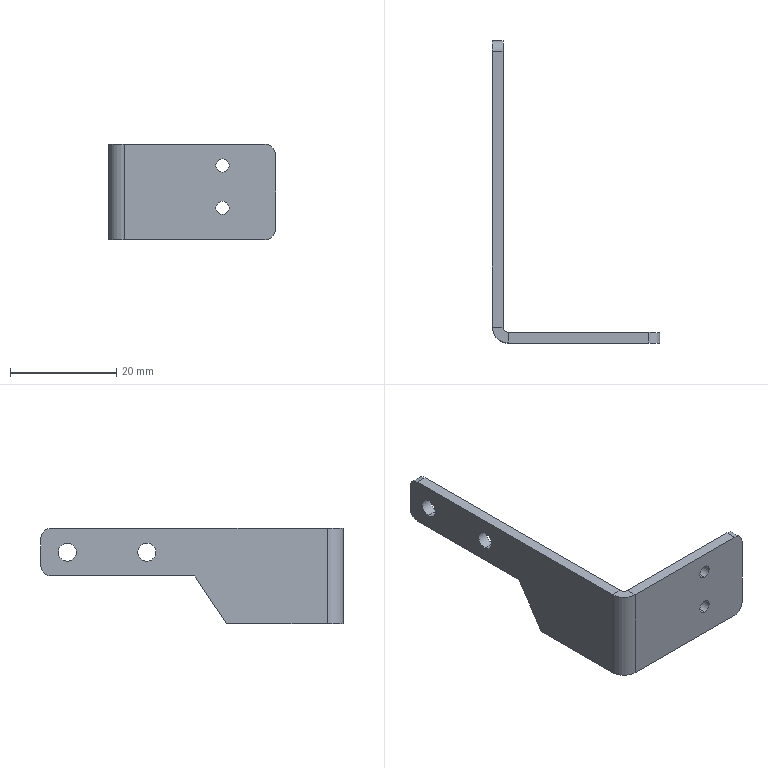Part | NX | features BREP 1 | 1 solid | 28 faces | box 31.5 x 57 x 18 mm | volume 2444 mm3 | cylinder 14 | plane 14 | commonest cylinder face diameters 2.5 x4 3.4 x4 4 x4 2 x1 6 x1
STEP:
#1=CARTESIAN_POINT('',(-2.,50.,6.2));
#2=VERTEX_POINT('',#1);
#3=CARTESIAN_POINT('',(0.,50.,6.2));
#4=VERTEX_POINT('',#3);
#5=CARTESIAN_POINT('',(0.,50.,6.2));
#6=DIRECTION('',(1.,0.,0.));
#7=VECTOR('',#6,1000.);
#8=LINE('',#5,#7);
#9=EDGE_CURVE('',#2,#4,#8,.T.);
#10=ORIENTED_EDGE('',*,*,#9,.F.);
#11=CARTESIAN_POINT('',(-2.,50.,2.8));
#12=VERTEX_POINT('',#11);
#13=CARTESIAN_POINT('',(-2.,50.,4.5));
#14=DIRECTION('',(1.,0.,0.));
#15=DIRECTION('',(0.,0.,-1.));
#16=AXIS2_PLACEMENT_3D('',#13,#14,#15);
#17=CIRCLE('',#16,1.7);
#18=EDGE_CURVE('',#12,#2,#17,.T.);
#19=ORIENTED_EDGE('',*,*,#18,.F.);
#20=CARTESIAN_POINT('',(0.,50.,2.8));
#21=VERTEX_POINT('',#20);
#22=CARTESIAN_POINT('',(0.,50.,2.8));
#23=DIRECTION('',(1.,0.,0.));
#24=VECTOR('',#23,1000.);
#25=LINE('',#22,#24);
#26=EDGE_CURVE('',#12,#21,#25,.T.);
#27=ORIENTED_EDGE('',*,*,#26,.T.);
#28=CARTESIAN_POINT('',(0.,50.,4.5));
#29=DIRECTION('',(1.,0.,0.));
#30=DIRECTION('',(0.,0.,-1.));
#31=AXIS2_PLACEMENT_3D('',#28,#29,#30);
#32=CIRCLE('',#31,1.7);
#33=EDGE_CURVE('',#21,#4,#32,.T.);
#34=ORIENTED_EDGE('',*,*,#33,.T.);
#35=EDGE_LOOP('',(#10,#19,#27,#34));
#36=FACE_BOUND('',#35,.T.);
#37=CARTESIAN_POINT('',(0.,50.,4.5));
#38=DIRECTION('',(1.,0.,0.));
#39=DIRECTION('',(0.,0.,-1.));
#40=AXIS2_PLACEMENT_3D('',#37,#38,#39);
#41=CYLINDRICAL_SURFACE('',#40,1.7);
#42=ADVANCED_FACE('',(#36),#41,.F.);
#43=CARTESIAN_POINT('',(-2.,35.,6.2));
#44=VERTEX_POINT('',#43);
#45=CARTESIAN_POINT('',(0.,35.,6.2));
#46=VERTEX_POINT('',#45);
#47=CARTESIAN_POINT('',(0.,35.,6.2));
#48=DIRECTION('',(1.,0.,0.));
#49=VECTOR('',#48,1000.);
#50=LINE('',#47,#49);
#51=EDGE_CURVE('',#44,#46,#50,.T.);
#52=ORIENTED_EDGE('',*,*,#51,.F.);
#53=CARTESIAN_POINT('',(-2.,35.,2.8));
#54=VERTEX_POINT('',#53);
#55=CARTESIAN_POINT('',(-2.,35.,4.5));
#56=DIRECTION('',(1.,0.,0.));
#57=DIRECTION('',(0.,0.,-1.));
#58=AXIS2_PLACEMENT_3D('',#55,#56,#57);
#59=CIRCLE('',#58,1.7);
#60=EDGE_CURVE('',#54,#44,#59,.T.);
#61=ORIENTED_EDGE('',*,*,#60,.F.);
#62=CARTESIAN_POINT('',(0.,35.,2.8));
#63=VERTEX_POINT('',#62);
#64=CARTESIAN_POINT('',(0.,35.,2.8));
#65=DIRECTION('',(1.,0.,0.));
#66=VECTOR('',#65,1000.);
#67=LINE('',#64,#66);
#68=EDGE_CURVE('',#54,#63,#67,.T.);
#69=ORIENTED_EDGE('',*,*,#68,.T.);
#70=CARTESIAN_POINT('',(0.,35.,4.5));
#71=DIRECTION('',(1.,0.,0.));
#72=DIRECTION('',(0.,0.,-1.));
#73=AXIS2_PLACEMENT_3D('',#70,#71,#72);
#74=CIRCLE('',#73,1.7);
#75=EDGE_CURVE('',#63,#46,#74,.T.);
#76=ORIENTED_EDGE('',*,*,#75,.T.);
#77=EDGE_LOOP('',(#52,#61,#69,#76));
#78=FACE_BOUND('',#77,.T.);
#79=CARTESIAN_POINT('',(0.,35.,4.5));
#80=DIRECTION('',(1.,0.,0.));
#81=DIRECTION('',(0.,0.,-1.));
#82=AXIS2_PLACEMENT_3D('',#79,#80,#81);
#83=CYLINDRICAL_SURFACE('',#82,1.7);
#84=ADVANCED_FACE('',(#78),#83,.F.);
#85=CARTESIAN_POINT('',(19.5,0.,-1.75));
#86=VERTEX_POINT('',#85);
#87=CARTESIAN_POINT('',(19.5,-2.,-1.75));
#88=VERTEX_POINT('',#87);
#89=CARTESIAN_POINT('',(19.5,-2.,-1.75));
#90=DIRECTION('',(0.,-1.,0.));
#91=VECTOR('',#90,1000.);
#92=LINE('',#89,#91);
#93=EDGE_CURVE('',#86,#88,#92,.T.);
#94=ORIENTED_EDGE('',*,*,#93,.F.);
#95=CARTESIAN_POINT('',(19.5,0.,-4.25));
#96=VERTEX_POINT('',#95);
#97=CARTESIAN_POINT('',(19.5,0.,-3.));
#98=DIRECTION('',(0.,1.,0.));
#99=DIRECTION('',(0.,0.,1.));
#100=AXIS2_PLACEMENT_3D('',#97,#98,#99);
#101=CIRCLE('',#100,1.25);
#102=EDGE_CURVE('',#86,#96,#101,.T.);
#103=ORIENTED_EDGE('',*,*,#102,.T.);
#104=CARTESIAN_POINT('',(19.5,-2.,-4.25));
#105=VERTEX_POINT('',#104);
#106=CARTESIAN_POINT('',(19.5,-2.,-4.25));
#107=DIRECTION('',(0.,-1.,0.));
#108=VECTOR('',#107,1000.);
#109=LINE('',#106,#108);
#110=EDGE_CURVE('',#96,#105,#109,.T.);
#111=ORIENTED_EDGE('',*,*,#110,.T.);
#112=CARTESIAN_POINT('',(19.5,-2.,-3.));
#113=DIRECTION('',(0.,-1.,0.));
#114=DIRECTION('',(0.,0.,-1.));
#115=AXIS2_PLACEMENT_3D('',#112,#113,#114);
#116=CIRCLE('',#115,1.25);
#117=EDGE_CURVE('',#105,#88,#116,.T.);
#118=ORIENTED_EDGE('',*,*,#117,.T.);
#119=EDGE_LOOP('',(#94,#103,#111,#118));
#120=FACE_BOUND('',#119,.T.);
#121=CARTESIAN_POINT('',(19.5,-2.,-3.));
#122=DIRECTION('',(0.,-1.,0.));
#123=DIRECTION('',(0.,0.,-1.));
#124=AXIS2_PLACEMENT_3D('',#121,#122,#123);
#125=CYLINDRICAL_SURFACE('',#124,1.25);
#126=ADVANCED_FACE('',(#120),#125,.F.);
#127=CARTESIAN_POINT('',(19.5,0.,6.25));
#128=VERTEX_POINT('',#127);
#129=CARTESIAN_POINT('',(19.5,-2.,6.25));
#130=VERTEX_POINT('',#129);
#131=CARTESIAN_POINT('',(19.5,-2.,6.25));
#132=DIRECTION('',(0.,-1.,0.));
#133=VECTOR('',#132,1000.);
#134=LINE('',#131,#133);
#135=EDGE_CURVE('',#128,#130,#134,.T.);
#136=ORIENTED_EDGE('',*,*,#135,.F.);
#137=CARTESIAN_POINT('',(19.5,0.,3.75));
#138=VERTEX_POINT('',#137);
#139=CARTESIAN_POINT('',(19.5,0.,5.));
#140=DIRECTION('',(0.,1.,0.));
#141=DIRECTION('',(0.,0.,1.));
#142=AXIS2_PLACEMENT_3D('',#139,#140,#141);
#143=CIRCLE('',#142,1.25);
#144=EDGE_CURVE('',#128,#138,#143,.T.);
#145=ORIENTED_EDGE('',*,*,#144,.T.);
#146=CARTESIAN_POINT('',(19.5,-2.,3.75));
#147=VERTEX_POINT('',#146);
#148=CARTESIAN_POINT('',(19.5,-2.,3.75));
#149=DIRECTION('',(0.,-1.,0.));
#150=VECTOR('',#149,1000.);
#151=LINE('',#148,#150);
#152=EDGE_CURVE('',#138,#147,#151,.T.);
#153=ORIENTED_EDGE('',*,*,#152,.T.);
#154=CARTESIAN_POINT('',(19.5,-2.,5.));
#155=DIRECTION('',(0.,-1.,0.));
#156=DIRECTION('',(0.,0.,-1.));
#157=AXIS2_PLACEMENT_3D('',#154,#155,#156);
#158=CIRCLE('',#157,1.25);
#159=EDGE_CURVE('',#147,#130,#158,.T.);
#160=ORIENTED_EDGE('',*,*,#159,.T.);
#161=EDGE_LOOP('',(#136,#145,#153,#160));
#162=FACE_BOUND('',#161,.T.);
#163=CARTESIAN_POINT('',(19.5,-2.,5.));
#164=DIRECTION('',(0.,-1.,0.));
#165=DIRECTION('',(0.,0.,-1.));
#166=AXIS2_PLACEMENT_3D('',#163,#164,#165);
#167=CYLINDRICAL_SURFACE('',#166,1.25);
#168=ADVANCED_FACE('',(#162),#167,.F.);
#169=CARTESIAN_POINT('',(-2.,53.,9.));
#170=VERTEX_POINT('',#169);
#171=CARTESIAN_POINT('',(-2.,55.,7.));
#172=VERTEX_POINT('',#171);
#173=CARTESIAN_POINT('',(-2.,53.,7.));
#174=DIRECTION('',(-1.,0.,0.));
#175=DIRECTION('',(0.,1.,0.));
#176=AXIS2_PLACEMENT_3D('',#173,#174,#175);
#177=CIRCLE('',#176,2.);
#178=EDGE_CURVE('',#170,#172,#177,.T.);
#179=ORIENTED_EDGE('',*,*,#178,.F.);
#180=CARTESIAN_POINT('',(0.,53.,9.));
#181=VERTEX_POINT('',#180);
#182=CARTESIAN_POINT('',(-2.,53.,9.));
#183=DIRECTION('',(-1.,0.,0.));
#184=VECTOR('',#183,1000.);
#185=LINE('',#182,#184);
#186=EDGE_CURVE('',#181,#170,#185,.T.);
#187=ORIENTED_EDGE('',*,*,#186,.F.);
#188=CARTESIAN_POINT('',(0.,55.,7.));
#189=VERTEX_POINT('',#188);
#190=CARTESIAN_POINT('',(0.,53.,7.));
#191=DIRECTION('',(1.,0.,0.));
#192=DIRECTION('',(0.,1.,0.));
#193=AXIS2_PLACEMENT_3D('',#190,#191,#192);
#194=CIRCLE('',#193,2.);
#195=EDGE_CURVE('',#189,#181,#194,.T.);
#196=ORIENTED_EDGE('',*,*,#195,.F.);
#197=CARTESIAN_POINT('',(0.,55.,7.));
#198=DIRECTION('',(1.,0.,0.));
#199=VECTOR('',#198,1000.);
#200=LINE('',#197,#199);
#201=EDGE_CURVE('',#172,#189,#200,.T.);
#202=ORIENTED_EDGE('',*,*,#201,.F.);
#203=EDGE_LOOP('',(#179,#187,#196,#202));
#204=FACE_BOUND('',#203,.T.);
#205=CARTESIAN_POINT('',(-2.,53.,7.));
#206=DIRECTION('',(-1.,0.,0.));
#207=DIRECTION('',(0.,0.,1.));
#208=AXIS2_PLACEMENT_3D('',#205,#206,#207);
#209=CYLINDRICAL_SURFACE('',#208,2.);
#210=ADVANCED_FACE('',(#204),#209,.T.);
#211=CARTESIAN_POINT('',(27.5,0.,9.));
#212=VERTEX_POINT('',#211);
#213=CARTESIAN_POINT('',(29.5,0.,7.));
#214=VERTEX_POINT('',#213);
#215=CARTESIAN_POINT('',(27.5,0.,7.));
#216=DIRECTION('',(0.,1.,0.));
#217=DIRECTION('',(0.,0.,1.));
#218=AXIS2_PLACEMENT_3D('',#215,#216,#217);
#219=CIRCLE('',#218,2.);
#220=EDGE_CURVE('',#212,#214,#219,.T.);
#221=ORIENTED_EDGE('',*,*,#220,.F.);
#222=CARTESIAN_POINT('',(27.5,-2.,9.));
#223=VERTEX_POINT('',#222);
#224=CARTESIAN_POINT('',(27.5,1.,9.));
#225=DIRECTION('',(0.,1.,0.));
#226=VECTOR('',#225,1000.);
#227=LINE('',#224,#226);
#228=EDGE_CURVE('',#223,#212,#227,.T.);
#229=ORIENTED_EDGE('',*,*,#228,.F.);
#230=CARTESIAN_POINT('',(29.5,-2.,7.));
#231=VERTEX_POINT('',#230);
#232=CARTESIAN_POINT('',(27.5,-2.,7.));
#233=DIRECTION('',(0.,-1.,0.));
#234=DIRECTION('',(0.,0.,1.));
#235=AXIS2_PLACEMENT_3D('',#232,#233,#234);
#236=CIRCLE('',#235,2.);
#237=EDGE_CURVE('',#231,#223,#236,.T.);
#238=ORIENTED_EDGE('',*,*,#237,.F.);
#239=CARTESIAN_POINT('',(29.5,0.,7.));
#240=DIRECTION('',(0.,-1.,0.));
#241=VECTOR('',#240,1000.);
#242=LINE('',#239,#241);
#243=EDGE_CURVE('',#214,#231,#242,.T.);
#244=ORIENTED_EDGE('',*,*,#243,.F.);
#245=EDGE_LOOP('',(#221,#229,#238,#244));
#246=FACE_BOUND('',#245,.T.);
#247=CARTESIAN_POINT('',(27.5,0.,7.));
#248=DIRECTION('',(0.,-1.,0.));
#249=DIRECTION('',(0.,0.,-1.));
#250=AXIS2_PLACEMENT_3D('',#247,#248,#249);
#251=CYLINDRICAL_SURFACE('',#250,2.);
#252=ADVANCED_FACE('',(#246),#251,.T.);
#253=CARTESIAN_POINT('',(29.5,0.,-7.));
#254=VERTEX_POINT('',#253);
#255=CARTESIAN_POINT('',(27.5,0.,-9.));
#256=VERTEX_POINT('',#255);
#257=CARTESIAN_POINT('',(27.5,0.,-7.));
#258=DIRECTION('',(0.,1.,0.));
#259=DIRECTION('',(0.,0.,1.));
#260=AXIS2_PLACEMENT_3D('',#257,#258,#259);
#261=CIRCLE('',#260,2.);
#262=EDGE_CURVE('',#254,#256,#261,.T.);
#263=ORIENTED_EDGE('',*,*,#262,.F.);
#264=CARTESIAN_POINT('',(29.5,-2.,-7.));
#265=VERTEX_POINT('',#264);
#266=CARTESIAN_POINT('',(29.5,0.,-7.));
#267=DIRECTION('',(0.,1.,0.));
#268=VECTOR('',#267,1000.);
#269=LINE('',#266,#268);
#270=EDGE_CURVE('',#265,#254,#269,.T.);
#271=ORIENTED_EDGE('',*,*,#270,.F.);
#272=CARTESIAN_POINT('',(27.5,-2.,-9.));
#273=VERTEX_POINT('',#272);
#274=CARTESIAN_POINT('',(27.5,-2.,-7.));
#275=DIRECTION('',(0.,-1.,0.));
#276=DIRECTION('',(0.,0.,1.));
#277=AXIS2_PLACEMENT_3D('',#274,#275,#276);
#278=CIRCLE('',#277,2.);
#279=EDGE_CURVE('',#273,#265,#278,.T.);
#280=ORIENTED_EDGE('',*,*,#279,.F.);
#281=CARTESIAN_POINT('',(27.5,1.,-9.));
#282=DIRECTION('',(0.,-1.,0.));
#283=VECTOR('',#282,1000.);
#284=LINE('',#281,#283);
#285=EDGE_CURVE('',#256,#273,#284,.T.);
#286=ORIENTED_EDGE('',*,*,#285,.F.);
#287=EDGE_LOOP('',(#263,#271,#280,#286));
#288=FACE_BOUND('',#287,.T.);
#289=CARTESIAN_POINT('',(27.5,1.,-7.));
#290=DIRECTION('',(0.,-1.,0.));
#291=DIRECTION('',(0.,0.,-1.));
#292=AXIS2_PLACEMENT_3D('',#289,#290,#291);
#293=CYLINDRICAL_SURFACE('',#292,2.);
#294=ADVANCED_FACE('',(#288),#293,.T.);
#295=CARTESIAN_POINT('',(0.,53.,0.));
#296=VERTEX_POINT('',#295);
#297=CARTESIAN_POINT('',(0.,55.,2.));
#298=VERTEX_POINT('',#297);
#299=CARTESIAN_POINT('',(0.,53.,2.));
#300=DIRECTION('',(1.,0.,0.));
#301=DIRECTION('',(0.,1.,0.));
#302=AXIS2_PLACEMENT_3D('',#299,#300,#301);
#303=CIRCLE('',#302,2.);
#304=EDGE_CURVE('',#296,#298,#303,.T.);
#305=ORIENTED_EDGE('',*,*,#304,.F.);
#306=CARTESIAN_POINT('',(-2.,53.,0.));
#307=VERTEX_POINT('',#306);
#308=CARTESIAN_POINT('',(0.,53.,0.));
#309=DIRECTION('',(1.,0.,0.));
#310=VECTOR('',#309,1000.);
#311=LINE('',#308,#310);
#312=EDGE_CURVE('',#307,#296,#311,.T.);
#313=ORIENTED_EDGE('',*,*,#312,.F.);
#314=CARTESIAN_POINT('',(-2.,55.,2.));
#315=VERTEX_POINT('',#314);
#316=CARTESIAN_POINT('',(-2.,53.,2.));
#317=DIRECTION('',(-1.,0.,0.));
#318=DIRECTION('',(0.,1.,0.));
#319=AXIS2_PLACEMENT_3D('',#316,#317,#318);
#320=CIRCLE('',#319,2.);
#321=EDGE_CURVE('',#315,#307,#320,.T.);
#322=ORIENTED_EDGE('',*,*,#321,.F.);
#323=CARTESIAN_POINT('',(-2.,55.,2.));
#324=DIRECTION('',(-1.,0.,0.));
#325=VECTOR('',#324,1000.);
#326=LINE('',#323,#325);
#327=EDGE_CURVE('',#298,#315,#326,.T.);
#328=ORIENTED_EDGE('',*,*,#327,.F.);
#329=EDGE_LOOP('',(#305,#313,#322,#328));
#330=FACE_BOUND('',#329,.T.);
#331=CARTESIAN_POINT('',(-2.,53.,2.));
#332=DIRECTION('',(-1.,0.,0.));
#333=DIRECTION('',(0.,0.,1.));
#334=AXIS2_PLACEMENT_3D('',#331,#332,#333);
#335=CYLINDRICAL_SURFACE('',#334,2.);
#336=ADVANCED_FACE('',(#330),#335,.T.);
#337=CARTESIAN_POINT('',(0.,26.,0.));
#338=VERTEX_POINT('',#337);
#339=CARTESIAN_POINT('',(0.,20.,-9.));
#340=VERTEX_POINT('',#339);
#341=CARTESIAN_POINT('',(0.,39.077,19.615));
#342=DIRECTION('',(0.,-0.5547,-0.8321));
#343=VECTOR('',#342,1000.);
#344=LINE('',#341,#343);
#345=EDGE_CURVE('',#338,#340,#344,.T.);
#346=ORIENTED_EDGE('',*,*,#345,.T.);
#347=CARTESIAN_POINT('',(-2.,20.,-9.));
#348=VERTEX_POINT('',#347);
#349=CARTESIAN_POINT('',(0.,20.,-9.));
#350=DIRECTION('',(-1.,0.,0.));
#351=VECTOR('',#350,1000.);
#352=LINE('',#349,#351);
#353=EDGE_CURVE('',#340,#348,#352,.T.);
#354=ORIENTED_EDGE('',*,*,#353,.T.);
#355=CARTESIAN_POINT('',(-2.,26.,0.));
#356=VERTEX_POINT('',#355);
#357=CARTESIAN_POINT('',(-2.,39.077,19.615));
#358=DIRECTION('',(0.,-0.5547,-0.8321));
#359=VECTOR('',#358,1000.);
#360=LINE('',#357,#359);
#361=EDGE_CURVE('',#356,#348,#360,.T.);
#362=ORIENTED_EDGE('',*,*,#361,.F.);
#363=CARTESIAN_POINT('',(0.,26.,0.));
#364=DIRECTION('',(-1.,0.,0.));
#365=VECTOR('',#364,1000.);
#366=LINE('',#363,#365);
#367=EDGE_CURVE('',#338,#356,#366,.T.);
#368=ORIENTED_EDGE('',*,*,#367,.F.);
#369=EDGE_LOOP('',(#346,#354,#362,#368));
#370=FACE_BOUND('',#369,.T.);
#371=CARTESIAN_POINT('',(0.,39.077,19.615));
#372=DIRECTION('',(0.,-0.8321,0.5547));
#373=DIRECTION('',(0.,-0.5547,-0.8321));
#374=AXIS2_PLACEMENT_3D('',#371,#372,#373);
#375=PLANE('',#374);
#376=ADVANCED_FACE('',(#370),#375,.F.);
#377=CARTESIAN_POINT('',(-2.,55.,0.));
#378=DIRECTION('',(0.,1.,0.));
#379=VECTOR('',#378,1000.);
#380=LINE('',#377,#379);
#381=EDGE_CURVE('',#356,#307,#380,.T.);
#382=ORIENTED_EDGE('',*,*,#381,.T.);
#383=ORIENTED_EDGE('',*,*,#312,.T.);
#384=CARTESIAN_POINT('',(0.,55.,0.));
#385=DIRECTION('',(0.,1.,0.));
#386=VECTOR('',#385,1000.);
#387=LINE('',#384,#386);
#388=EDGE_CURVE('',#338,#296,#387,.T.);
#389=ORIENTED_EDGE('',*,*,#388,.F.);
#390=ORIENTED_EDGE('',*,*,#367,.T.);
#391=EDGE_LOOP('',(#382,#383,#389,#390));
#392=FACE_BOUND('',#391,.T.);
#393=CARTESIAN_POINT('',(0.,55.,0.));
#394=DIRECTION('',(0.,0.,-1.));
#395=DIRECTION('',(0.,1.,0.));
#396=AXIS2_PLACEMENT_3D('',#393,#394,#395);
#397=PLANE('',#396);
#398=ADVANCED_FACE('',(#392),#397,.T.);
#399=CARTESIAN_POINT('',(1.,0.,-9.));
#400=VERTEX_POINT('',#399);
#401=CARTESIAN_POINT('',(0.,0.,-9.));
#402=DIRECTION('',(1.,0.,0.));
#403=VECTOR('',#402,1000.);
#404=LINE('',#401,#403);
#405=EDGE_CURVE('',#400,#256,#404,.T.);
#406=ORIENTED_EDGE('',*,*,#405,.T.);
#407=ORIENTED_EDGE('',*,*,#285,.T.);
#408=CARTESIAN_POINT('',(1.,-2.,-9.));
#409=VERTEX_POINT('',#408);
#410=CARTESIAN_POINT('',(0.,-2.,-9.));
#411=DIRECTION('',(1.,0.,0.));
#412=VECTOR('',#411,1000.);
#413=LINE('',#410,#412);
#414=EDGE_CURVE('',#409,#273,#413,.T.);
#415=ORIENTED_EDGE('',*,*,#414,.F.);
#416=CARTESIAN_POINT('',(1.,-2.,-9.));
#417=DIRECTION('',(0.,1.,0.));
#418=VECTOR('',#417,1000.);
#419=LINE('',#416,#418);
#420=EDGE_CURVE('',#409,#400,#419,.T.);
#421=ORIENTED_EDGE('',*,*,#420,.T.);
#422=EDGE_LOOP('',(#406,#407,#415,#421));
#423=FACE_BOUND('',#422,.T.);
#424=CARTESIAN_POINT('',(1.,1.,-9.));
#425=DIRECTION('',(0.,0.,-1.));
#426=DIRECTION('',(-1.,0.,0.));
#427=AXIS2_PLACEMENT_3D('',#424,#425,#426);
#428=PLANE('',#427);
#429=ADVANCED_FACE('',(#423),#428,.T.);
#430=CARTESIAN_POINT('',(0.,1.,9.));
#431=VERTEX_POINT('',#430);
#432=CARTESIAN_POINT('',(0.,55.,9.));
#433=DIRECTION('',(0.,-1.,0.));
#434=VECTOR('',#433,1000.);
#435=LINE('',#432,#434);
#436=EDGE_CURVE('',#181,#431,#435,.T.);
#437=ORIENTED_EDGE('',*,*,#436,.F.);
#438=ORIENTED_EDGE('',*,*,#186,.T.);
#439=CARTESIAN_POINT('',(-2.,1.,9.));
#440=VERTEX_POINT('',#439);
#441=CARTESIAN_POINT('',(-2.,55.,9.));
#442=DIRECTION('',(0.,-1.,0.));
#443=VECTOR('',#442,1000.);
#444=LINE('',#441,#443);
#445=EDGE_CURVE('',#170,#440,#444,.T.);
#446=ORIENTED_EDGE('',*,*,#445,.T.);
#447=CARTESIAN_POINT('',(-2.,1.,9.));
#448=DIRECTION('',(1.,0.,0.));
#449=VECTOR('',#448,1000.);
#450=LINE('',#447,#449);
#451=EDGE_CURVE('',#440,#431,#450,.T.);
#452=ORIENTED_EDGE('',*,*,#451,.T.);
#453=EDGE_LOOP('',(#437,#438,#446,#452));
#454=FACE_BOUND('',#453,.T.);
#455=CARTESIAN_POINT('',(1.,1.,9.));
#456=DIRECTION('',(0.,0.,-1.));
#457=DIRECTION('',(-1.,0.,0.));
#458=AXIS2_PLACEMENT_3D('',#455,#456,#457);
#459=PLANE('',#458);
#460=ADVANCED_FACE('',(#454),#459,.F.);
#461=CARTESIAN_POINT('',(-2.,1.,-9.));
#462=VERTEX_POINT('',#461);
#463=CARTESIAN_POINT('',(1.,1.,-9.));
#464=DIRECTION('',(0.,0.,1.));
#465=DIRECTION('',(1.,0.,0.));
#466=AXIS2_PLACEMENT_3D('',#463,#464,#465);
#467=CIRCLE('',#466,3.);
#468=EDGE_CURVE('',#462,#409,#467,.T.);
#469=ORIENTED_EDGE('',*,*,#468,.T.);
#470=CARTESIAN_POINT('',(1.,-2.,9.));
#471=VERTEX_POINT('',#470);
#472=CARTESIAN_POINT('',(1.,-2.,9.));
#473=DIRECTION('',(0.,0.,-1.));
#474=VECTOR('',#473,1000.);
#475=LINE('',#472,#474);
#476=EDGE_CURVE('',#471,#409,#475,.T.);
#477=ORIENTED_EDGE('',*,*,#476,.F.);
#478=CARTESIAN_POINT('',(1.,1.,9.));
#479=DIRECTION('',(0.,0.,1.));
#480=DIRECTION('',(1.,0.,0.));
#481=AXIS2_PLACEMENT_3D('',#478,#479,#480);
#482=CIRCLE('',#481,3.);
#483=EDGE_CURVE('',#440,#471,#482,.T.);
#484=ORIENTED_EDGE('',*,*,#483,.F.);
#485=CARTESIAN_POINT('',(-2.,1.,9.));
#486=DIRECTION('',(0.,0.,-1.));
#487=VECTOR('',#486,1000.);
#488=LINE('',#485,#487);
#489=EDGE_CURVE('',#440,#462,#488,.T.);
#490=ORIENTED_EDGE('',*,*,#489,.T.);
#491=EDGE_LOOP('',(#469,#477,#484,#490));
#492=FACE_BOUND('',#491,.T.);
#493=CARTESIAN_POINT('',(1.,1.,9.));
#494=DIRECTION('',(0.,0.,-1.));
#495=DIRECTION('',(-1.,0.,0.));
#496=AXIS2_PLACEMENT_3D('',#493,#494,#495);
#497=CYLINDRICAL_SURFACE('',#496,3.);
#498=ADVANCED_FACE('',(#492),#497,.T.);
#499=CARTESIAN_POINT('',(0.,1.,-9.));
#500=VERTEX_POINT('',#499);
#501=CARTESIAN_POINT('',(1.,1.,-9.));
#502=DIRECTION('',(0.,0.,1.));
#503=DIRECTION('',(-1.,0.,0.));
#504=AXIS2_PLACEMENT_3D('',#501,#502,#503);
#505=CIRCLE('',#504,1.);
#506=EDGE_CURVE('',#500,#400,#505,.T.);
#507=ORIENTED_EDGE('',*,*,#506,.F.);
#508=CARTESIAN_POINT('',(0.,1.,9.));
#509=DIRECTION('',(0.,0.,-1.));
#510=VECTOR('',#509,1000.);
#511=LINE('',#508,#510);
#512=EDGE_CURVE('',#431,#500,#511,.T.);
#513=ORIENTED_EDGE('',*,*,#512,.F.);
#514=CARTESIAN_POINT('',(1.,0.,9.));
#515=VERTEX_POINT('',#514);
#516=CARTESIAN_POINT('',(1.,1.,9.));
#517=DIRECTION('',(0.,0.,1.));
#518=DIRECTION('',(-1.,0.,0.));
#519=AXIS2_PLACEMENT_3D('',#516,#517,#518);
#520=CIRCLE('',#519,1.);
#521=EDGE_CURVE('',#431,#515,#520,.T.);
#522=ORIENTED_EDGE('',*,*,#521,.T.);
#523=CARTESIAN_POINT('',(1.,0.,9.));
#524=DIRECTION('',(0.,0.,-1.));
#525=VECTOR('',#524,1000.);
#526=LINE('',#523,#525);
#527=EDGE_CURVE('',#515,#400,#526,.T.);
#528=ORIENTED_EDGE('',*,*,#527,.T.);
#529=EDGE_LOOP('',(#507,#513,#522,#528));
#530=FACE_BOUND('',#529,.T.);
#531=CARTESIAN_POINT('',(1.,1.,9.));
#532=DIRECTION('',(0.,0.,-1.));
#533=DIRECTION('',(-1.,0.,0.));
#534=AXIS2_PLACEMENT_3D('',#531,#532,#533);
#535=CYLINDRICAL_SURFACE('',#534,1.);
#536=ADVANCED_FACE('',(#530),#535,.F.);
#537=CARTESIAN_POINT('',(29.5,0.,9.));
#538=DIRECTION('',(0.,0.,-1.));
#539=VECTOR('',#538,1000.);
#540=LINE('',#537,#539);
#541=EDGE_CURVE('',#214,#254,#540,.T.);
#542=ORIENTED_EDGE('',*,*,#541,.T.);
#543=ORIENTED_EDGE('',*,*,#262,.T.);
#544=ORIENTED_EDGE('',*,*,#405,.F.);
#545=ORIENTED_EDGE('',*,*,#527,.F.);
#546=CARTESIAN_POINT('',(0.,0.,9.));
#547=DIRECTION('',(1.,0.,0.));
#548=VECTOR('',#547,1000.);
#549=LINE('',#546,#548);
#550=EDGE_CURVE('',#515,#212,#549,.T.);
#551=ORIENTED_EDGE('',*,*,#550,.T.);
#552=ORIENTED_EDGE('',*,*,#220,.T.);
#553=EDGE_LOOP('',(#542,#543,#544,#545,#551,#552));
#554=FACE_BOUND('',#553,.T.);
#555=CARTESIAN_POINT('',(19.5,0.,5.));
#556=DIRECTION('',(0.,1.,0.));
#557=DIRECTION('',(0.,0.,1.));
#558=AXIS2_PLACEMENT_3D('',#555,#556,#557);
#559=CIRCLE('',#558,1.25);
#560=EDGE_CURVE('',#138,#128,#559,.T.);
#561=ORIENTED_EDGE('',*,*,#560,.F.);
#562=ORIENTED_EDGE('',*,*,#144,.F.);
#563=EDGE_LOOP('',(#561,#562));
#564=FACE_BOUND('',#563,.T.);
#565=CARTESIAN_POINT('',(19.5,0.,-3.));
#566=DIRECTION('',(0.,1.,0.));
#567=DIRECTION('',(0.,0.,1.));
#568=AXIS2_PLACEMENT_3D('',#565,#566,#567);
#569=CIRCLE('',#568,1.25);
#570=EDGE_CURVE('',#96,#86,#569,.T.);
#571=ORIENTED_EDGE('',*,*,#570,.F.);
#572=ORIENTED_EDGE('',*,*,#102,.F.);
#573=EDGE_LOOP('',(#571,#572));
#574=FACE_BOUND('',#573,.T.);
#575=CARTESIAN_POINT('',(0.,0.,9.));
#576=DIRECTION('',(0.,1.,0.));
#577=DIRECTION('',(0.,0.,1.));
#578=AXIS2_PLACEMENT_3D('',#575,#576,#577);
#579=PLANE('',#578);
#580=ADVANCED_FACE('',(#554,#564,#574),#579,.T.);
#581=CARTESIAN_POINT('',(29.5,-2.,9.));
#582=DIRECTION('',(0.,0.,-1.));
#583=VECTOR('',#582,1000.);
#584=LINE('',#581,#583);
#585=EDGE_CURVE('',#231,#265,#584,.T.);
#586=ORIENTED_EDGE('',*,*,#585,.T.);
#587=ORIENTED_EDGE('',*,*,#270,.T.);
#588=ORIENTED_EDGE('',*,*,#541,.F.);
#589=ORIENTED_EDGE('',*,*,#243,.T.);
#590=EDGE_LOOP('',(#586,#587,#588,#589));
#591=FACE_BOUND('',#590,.T.);
#592=CARTESIAN_POINT('',(29.5,0.,9.));
#593=DIRECTION('',(1.,0.,0.));
#594=DIRECTION('',(0.,0.,-1.));
#595=AXIS2_PLACEMENT_3D('',#592,#593,#594);
#596=PLANE('',#595);
#597=ADVANCED_FACE('',(#591),#596,.T.);
#598=ORIENTED_EDGE('',*,*,#414,.T.);
#599=ORIENTED_EDGE('',*,*,#279,.T.);
#600=ORIENTED_EDGE('',*,*,#585,.F.);
#601=ORIENTED_EDGE('',*,*,#237,.T.);
#602=CARTESIAN_POINT('',(0.,-2.,9.));
#603=DIRECTION('',(1.,0.,0.));
#604=VECTOR('',#603,1000.);
#605=LINE('',#602,#604);
#606=EDGE_CURVE('',#471,#223,#605,.T.);
#607=ORIENTED_EDGE('',*,*,#606,.F.);
#608=ORIENTED_EDGE('',*,*,#476,.T.);
#609=EDGE_LOOP('',(#598,#599,#600,#601,#607,#608));
#610=FACE_BOUND('',#609,.T.);
#611=ORIENTED_EDGE('',*,*,#159,.F.);
#612=CARTESIAN_POINT('',(19.5,-2.,5.));
#613=DIRECTION('',(0.,-1.,0.));
#614=DIRECTION('',(0.,0.,-1.));
#615=AXIS2_PLACEMENT_3D('',#612,#613,#614);
#616=CIRCLE('',#615,1.25);
#617=EDGE_CURVE('',#130,#147,#616,.T.);
#618=ORIENTED_EDGE('',*,*,#617,.F.);
#619=EDGE_LOOP('',(#611,#618));
#620=FACE_BOUND('',#619,.T.);
#621=ORIENTED_EDGE('',*,*,#117,.F.);
#622=CARTESIAN_POINT('',(19.5,-2.,-3.));
#623=DIRECTION('',(0.,-1.,0.));
#624=DIRECTION('',(0.,0.,-1.));
#625=AXIS2_PLACEMENT_3D('',#622,#623,#624);
#626=CIRCLE('',#625,1.25);
#627=EDGE_CURVE('',#88,#105,#626,.T.);
#628=ORIENTED_EDGE('',*,*,#627,.F.);
#629=EDGE_LOOP('',(#621,#628));
#630=FACE_BOUND('',#629,.T.);
#631=CARTESIAN_POINT('',(0.,-2.,9.));
#632=DIRECTION('',(0.,1.,0.));
#633=DIRECTION('',(0.,0.,1.));
#634=AXIS2_PLACEMENT_3D('',#631,#632,#633);
#635=PLANE('',#634);
#636=ADVANCED_FACE('',(#610,#620,#630),#635,.F.);
#637=CARTESIAN_POINT('',(0.,1.,-9.));
#638=DIRECTION('',(-1.,0.,0.));
#639=VECTOR('',#638,1000.);
#640=LINE('',#637,#639);
#641=EDGE_CURVE('',#500,#462,#640,.T.);
#642=ORIENTED_EDGE('',*,*,#641,.F.);
#643=ORIENTED_EDGE('',*,*,#506,.T.);
#644=ORIENTED_EDGE('',*,*,#420,.F.);
#645=ORIENTED_EDGE('',*,*,#468,.F.);
#646=EDGE_LOOP('',(#642,#643,#644,#645));
#647=FACE_BOUND('',#646,.T.);
#648=CARTESIAN_POINT('',(0.,1.,-9.));
#649=DIRECTION('',(0.,0.,-1.));
#650=DIRECTION('',(-1.,0.,0.));
#651=AXIS2_PLACEMENT_3D('',#648,#649,#650);
#652=PLANE('',#651);
#653=ADVANCED_FACE('',(#647),#652,.T.);
#654=ORIENTED_EDGE('',*,*,#606,.T.);
#655=ORIENTED_EDGE('',*,*,#228,.T.);
#656=ORIENTED_EDGE('',*,*,#550,.F.);
#657=CARTESIAN_POINT('',(1.,0.,9.));
#658=DIRECTION('',(0.,-1.,0.));
#659=VECTOR('',#658,1000.);
#660=LINE('',#657,#659);
#661=EDGE_CURVE('',#515,#471,#660,.T.);
#662=ORIENTED_EDGE('',*,*,#661,.T.);
#663=EDGE_LOOP('',(#654,#655,#656,#662));
#664=FACE_BOUND('',#663,.T.);
#665=CARTESIAN_POINT('',(-2.,1.,9.));
#666=DIRECTION('',(0.,0.,1.));
#667=DIRECTION('',(1.,0.,0.));
#668=AXIS2_PLACEMENT_3D('',#665,#666,#667);
#669=PLANE('',#668);
#670=ADVANCED_FACE('',(#664),#669,.T.);
#671=ORIENTED_EDGE('',*,*,#661,.F.);
#672=ORIENTED_EDGE('',*,*,#521,.F.);
#673=ORIENTED_EDGE('',*,*,#451,.F.);
#674=ORIENTED_EDGE('',*,*,#483,.T.);
#675=EDGE_LOOP('',(#671,#672,#673,#674));
#676=FACE_BOUND('',#675,.T.);
#677=CARTESIAN_POINT('',(1.,0.,9.));
#678=DIRECTION('',(0.,0.,1.));
#679=DIRECTION('',(1.,0.,0.));
#680=AXIS2_PLACEMENT_3D('',#677,#678,#679);
#681=PLANE('',#680);
#682=ADVANCED_FACE('',(#676),#681,.T.);
#683=CARTESIAN_POINT('',(-2.,55.,9.));
#684=DIRECTION('',(0.,0.,-1.));
#685=VECTOR('',#684,1000.);
#686=LINE('',#683,#685);
#687=EDGE_CURVE('',#172,#315,#686,.T.);
#688=ORIENTED_EDGE('',*,*,#687,.T.);
#689=ORIENTED_EDGE('',*,*,#321,.T.);
#690=ORIENTED_EDGE('',*,*,#381,.F.);
#691=ORIENTED_EDGE('',*,*,#361,.T.);
#692=CARTESIAN_POINT('',(-2.,55.,-9.));
#693=DIRECTION('',(0.,-1.,0.));
#694=VECTOR('',#693,1000.);
#695=LINE('',#692,#694);
#696=EDGE_CURVE('',#348,#462,#695,.T.);
#697=ORIENTED_EDGE('',*,*,#696,.T.);
#698=ORIENTED_EDGE('',*,*,#489,.F.);
#699=ORIENTED_EDGE('',*,*,#445,.F.);
#700=ORIENTED_EDGE('',*,*,#178,.T.);
#701=EDGE_LOOP('',(#688,#689,#690,#691,#697,#698,#699,#700));
#702=FACE_BOUND('',#701,.T.);
#703=ORIENTED_EDGE('',*,*,#60,.T.);
#704=CARTESIAN_POINT('',(-2.,35.,4.5));
#705=DIRECTION('',(1.,0.,0.));
#706=DIRECTION('',(0.,0.,-1.));
#707=AXIS2_PLACEMENT_3D('',#704,#705,#706);
#708=CIRCLE('',#707,1.7);
#709=EDGE_CURVE('',#44,#54,#708,.T.);
#710=ORIENTED_EDGE('',*,*,#709,.T.);
#711=EDGE_LOOP('',(#703,#710));
#712=FACE_BOUND('',#711,.T.);
#713=ORIENTED_EDGE('',*,*,#18,.T.);
#714=CARTESIAN_POINT('',(-2.,50.,4.5));
#715=DIRECTION('',(1.,0.,0.));
#716=DIRECTION('',(0.,0.,-1.));
#717=AXIS2_PLACEMENT_3D('',#714,#715,#716);
#718=CIRCLE('',#717,1.7);
#719=EDGE_CURVE('',#2,#12,#718,.T.);
#720=ORIENTED_EDGE('',*,*,#719,.T.);
#721=EDGE_LOOP('',(#713,#720));
#722=FACE_BOUND('',#721,.T.);
#723=CARTESIAN_POINT('',(-2.,55.,9.));
#724=DIRECTION('',(1.,0.,0.));
#725=DIRECTION('',(0.,1.,0.));
#726=AXIS2_PLACEMENT_3D('',#723,#724,#725);
#727=PLANE('',#726);
#728=ADVANCED_FACE('',(#702,#712,#722),#727,.F.);
#729=CARTESIAN_POINT('',(0.,55.,9.));
#730=DIRECTION('',(0.,0.,-1.));
#731=VECTOR('',#730,1000.);
#732=LINE('',#729,#731);
#733=EDGE_CURVE('',#189,#298,#732,.T.);
#734=ORIENTED_EDGE('',*,*,#733,.T.);
#735=ORIENTED_EDGE('',*,*,#327,.T.);
#736=ORIENTED_EDGE('',*,*,#687,.F.);
#737=ORIENTED_EDGE('',*,*,#201,.T.);
#738=EDGE_LOOP('',(#734,#735,#736,#737));
#739=FACE_BOUND('',#738,.T.);
#740=CARTESIAN_POINT('',(-2.,55.,9.));
#741=DIRECTION('',(0.,1.,0.));
#742=DIRECTION('',(0.,0.,1.));
#743=AXIS2_PLACEMENT_3D('',#740,#741,#742);
#744=PLANE('',#743);
#745=ADVANCED_FACE('',(#739),#744,.T.);
#746=ORIENTED_EDGE('',*,*,#388,.T.);
#747=ORIENTED_EDGE('',*,*,#304,.T.);
#748=ORIENTED_EDGE('',*,*,#733,.F.);
#749=ORIENTED_EDGE('',*,*,#195,.T.);
#750=ORIENTED_EDGE('',*,*,#436,.T.);
#751=ORIENTED_EDGE('',*,*,#512,.T.);
#752=CARTESIAN_POINT('',(0.,55.,-9.));
#753=DIRECTION('',(0.,-1.,0.));
#754=VECTOR('',#753,1000.);
#755=LINE('',#752,#754);
#756=EDGE_CURVE('',#340,#500,#755,.T.);
#757=ORIENTED_EDGE('',*,*,#756,.F.);
#758=ORIENTED_EDGE('',*,*,#345,.F.);
#759=EDGE_LOOP('',(#746,#747,#748,#749,#750,#751,#757,#758));
#760=FACE_BOUND('',#759,.T.);
#761=ORIENTED_EDGE('',*,*,#75,.F.);
#762=CARTESIAN_POINT('',(0.,35.,4.5));
#763=DIRECTION('',(1.,0.,0.));
#764=DIRECTION('',(0.,0.,-1.));
#765=AXIS2_PLACEMENT_3D('',#762,#763,#764);
#766=CIRCLE('',#765,1.7);
#767=EDGE_CURVE('',#46,#63,#766,.T.);
#768=ORIENTED_EDGE('',*,*,#767,.F.);
#769=EDGE_LOOP('',(#761,#768));
#770=FACE_BOUND('',#769,.T.);
#771=ORIENTED_EDGE('',*,*,#33,.F.);
#772=CARTESIAN_POINT('',(0.,50.,4.5));
#773=DIRECTION('',(1.,0.,0.));
#774=DIRECTION('',(0.,0.,-1.));
#775=AXIS2_PLACEMENT_3D('',#772,#773,#774);
#776=CIRCLE('',#775,1.7);
#777=EDGE_CURVE('',#4,#21,#776,.T.);
#778=ORIENTED_EDGE('',*,*,#777,.F.);
#779=EDGE_LOOP('',(#771,#778));
#780=FACE_BOUND('',#779,.T.);
#781=CARTESIAN_POINT('',(0.,55.,9.));
#782=DIRECTION('',(1.,0.,0.));
#783=DIRECTION('',(0.,1.,0.));
#784=AXIS2_PLACEMENT_3D('',#781,#782,#783);
#785=PLANE('',#784);
#786=ADVANCED_FACE('',(#760,#770,#780),#785,.T.);
#787=ORIENTED_EDGE('',*,*,#696,.F.);
#788=ORIENTED_EDGE('',*,*,#353,.F.);
#789=ORIENTED_EDGE('',*,*,#756,.T.);
#790=ORIENTED_EDGE('',*,*,#641,.T.);
#791=EDGE_LOOP('',(#787,#788,#789,#790));
#792=FACE_BOUND('',#791,.T.);
#793=CARTESIAN_POINT('',(1.,-2.,-9.));
#794=DIRECTION('',(0.,0.,-1.));
#795=DIRECTION('',(-1.,0.,0.));
#796=AXIS2_PLACEMENT_3D('',#793,#794,#795);
#797=PLANE('',#796);
#798=ADVANCED_FACE('',(#792),#797,.T.);
#799=ORIENTED_EDGE('',*,*,#560,.T.);
#800=ORIENTED_EDGE('',*,*,#135,.T.);
#801=ORIENTED_EDGE('',*,*,#617,.T.);
#802=ORIENTED_EDGE('',*,*,#152,.F.);
#803=EDGE_LOOP('',(#799,#800,#801,#802));
#804=FACE_BOUND('',#803,.T.);
#805=CARTESIAN_POINT('',(19.5,-2.,5.));
#806=DIRECTION('',(0.,-1.,0.));
#807=DIRECTION('',(0.,0.,-1.));
#808=AXIS2_PLACEMENT_3D('',#805,#806,#807);
#809=CYLINDRICAL_SURFACE('',#808,1.25);
#810=ADVANCED_FACE('',(#804),#809,.F.);
#811=ORIENTED_EDGE('',*,*,#570,.T.);
#812=ORIENTED_EDGE('',*,*,#93,.T.);
#813=ORIENTED_EDGE('',*,*,#627,.T.);
#814=ORIENTED_EDGE('',*,*,#110,.F.);
#815=EDGE_LOOP('',(#811,#812,#813,#814));
#816=FACE_BOUND('',#815,.T.);
#817=CARTESIAN_POINT('',(19.5,-2.,-3.));
#818=DIRECTION('',(0.,-1.,0.));
#819=DIRECTION('',(0.,0.,-1.));
#820=AXIS2_PLACEMENT_3D('',#817,#818,#819);
#821=CYLINDRICAL_SURFACE('',#820,1.25);
#822=ADVANCED_FACE('',(#816),#821,.F.);
#823=ORIENTED_EDGE('',*,*,#709,.F.);
#824=ORIENTED_EDGE('',*,*,#51,.T.);
#825=ORIENTED_EDGE('',*,*,#767,.T.);
#826=ORIENTED_EDGE('',*,*,#68,.F.);
#827=EDGE_LOOP('',(#823,#824,#825,#826));
#828=FACE_BOUND('',#827,.T.);
#829=CARTESIAN_POINT('',(0.,35.,4.5));
#830=DIRECTION('',(1.,0.,0.));
#831=DIRECTION('',(0.,0.,-1.));
#832=AXIS2_PLACEMENT_3D('',#829,#830,#831);
#833=CYLINDRICAL_SURFACE('',#832,1.7);
#834=ADVANCED_FACE('',(#828),#833,.F.);
#835=ORIENTED_EDGE('',*,*,#719,.F.);
#836=ORIENTED_EDGE('',*,*,#9,.T.);
#837=ORIENTED_EDGE('',*,*,#777,.T.);
#838=ORIENTED_EDGE('',*,*,#26,.F.);
#839=EDGE_LOOP('',(#835,#836,#837,#838));
#840=FACE_BOUND('',#839,.T.);
#841=CARTESIAN_POINT('',(0.,50.,4.5));
#842=DIRECTION('',(1.,0.,0.));
#843=DIRECTION('',(0.,0.,-1.));
#844=AXIS2_PLACEMENT_3D('',#841,#842,#843);
#845=CYLINDRICAL_SURFACE('',#844,1.7);
#846=ADVANCED_FACE('',(#840),#845,.F.);
#847=CLOSED_SHELL('',(#42,#84,#126,#168,#210,#252,#294,#336,#376,#398,#429,#460,#498,#536,#580,#597,#636,#653,#670,#682,#728,#745,#786,#798,#810,#822,#834,#846));
#848=MANIFOLD_SOLID_BREP('',#847);
#849=(LENGTH_UNIT()NAMED_UNIT(*)SI_UNIT(.MILLI.,.METRE.));
#850=UNCERTAINTY_MEASURE_WITH_UNIT(LENGTH_MEASURE(0.00001),#849,'','');
#851=(NAMED_UNIT(*)PLANE_ANGLE_UNIT()SI_UNIT($,.RADIAN.));
#852=(NAMED_UNIT(*)SI_UNIT($,.STERADIAN.)SOLID_ANGLE_UNIT());
#853=(GEOMETRIC_REPRESENTATION_CONTEXT(3)GLOBAL_UNCERTAINTY_ASSIGNED_CONTEXT((#850))GLOBAL_UNIT_ASSIGNED_CONTEXT((#849,#851,#852))REPRESENTATION_CONTEXT('',''));
#854=ADVANCED_BREP_SHAPE_REPRESENTATION('',(#848),#853);